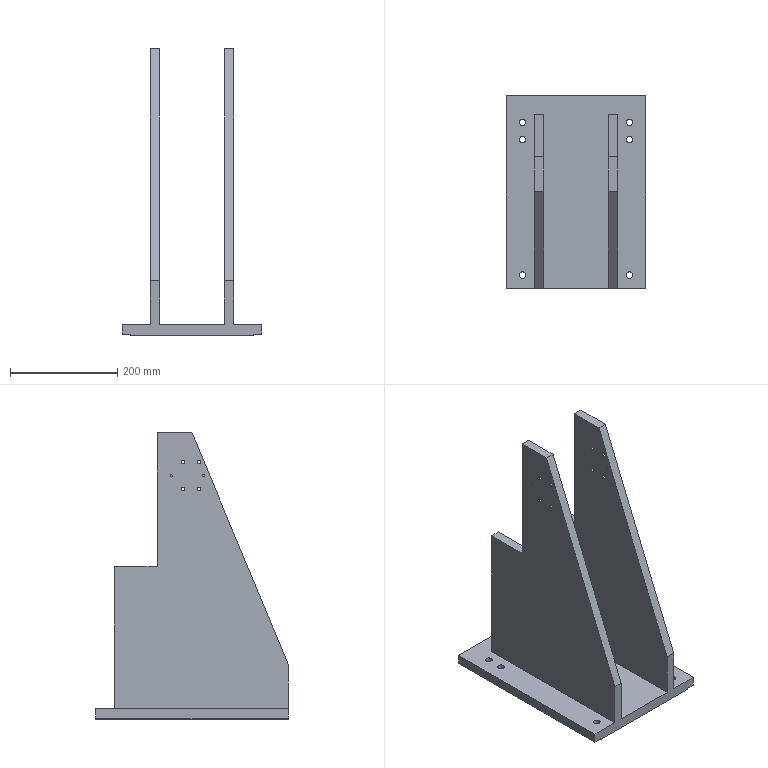Part | STEP file | MACHINE BASE PROJECTION 1 | 1 solid | 42 faces | box 260 x 360 x 535 mm | volume 5517318 mm3 | plane 24 | cylinder 18 | commonest cylinder face diameters 6.647 x8 12 x6 3.242 x4